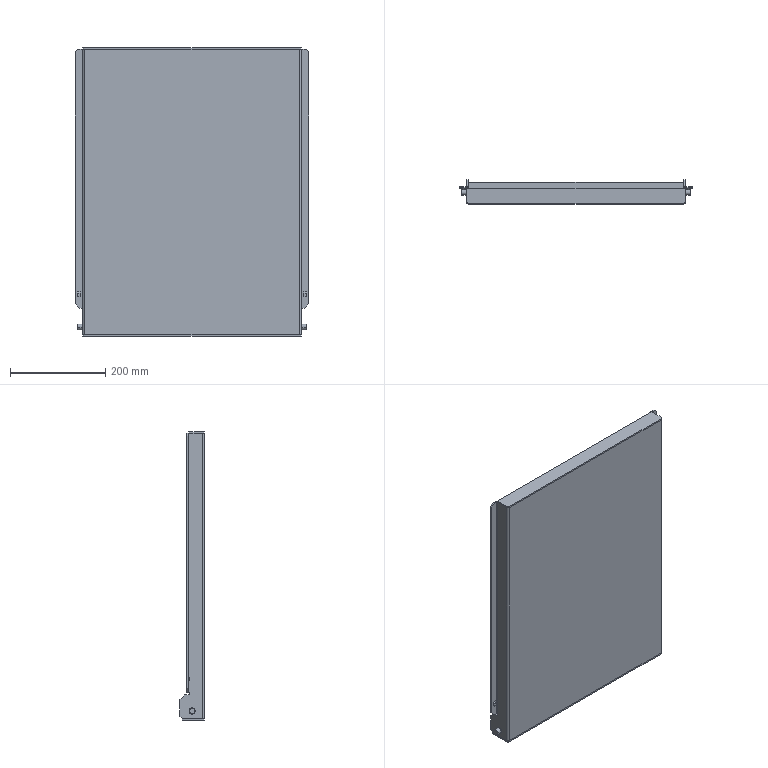Part | SolidWorks | features ICE 5, SM3dBend 4, Chamfer 2, Fillet 2, CosmeticWeldCutList 1, Extrusion 1, FlatPattern 1, MirrorPattern 1, SMBaseFlange 1, SheetMetal 1, SolidToSheetMetal 1 | 3 solids | 92 faces | box 491.996 x 51.073 x 606 mm | volume 1106182 mm3 | plane 72 | cylinder 20 | commonest cylinder face diameters 8 x8 2 x4 12 x4 13 x4